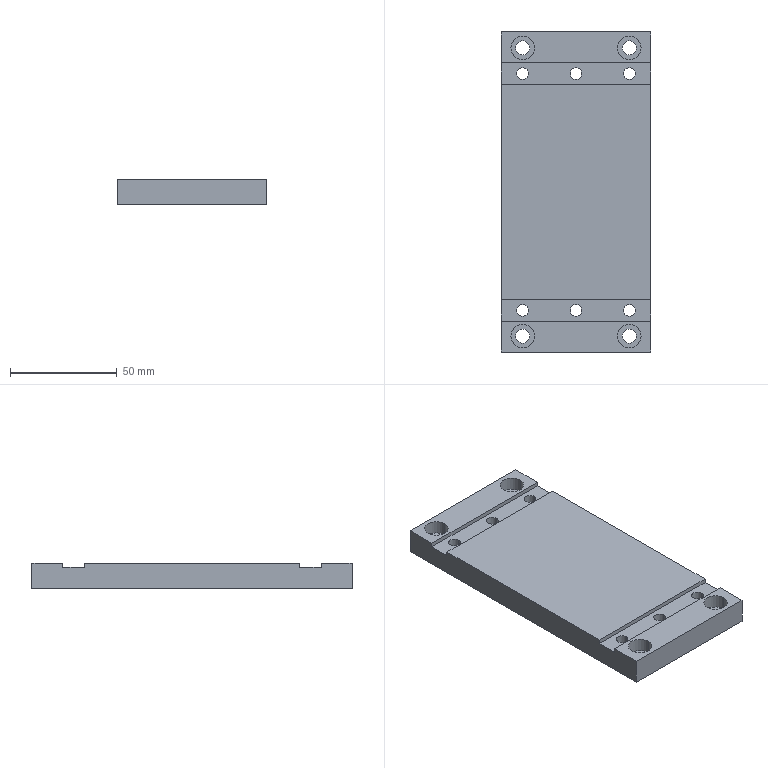Part | STEP file | C07 | 1 solid | 64 faces | box 70 x 150 x 12 mm | volume 116800 mm3 | cylinder 40 | plane 24 | commonest cylinder face diameters 5.5 x12 10 x12 6.6 x8 11 x8